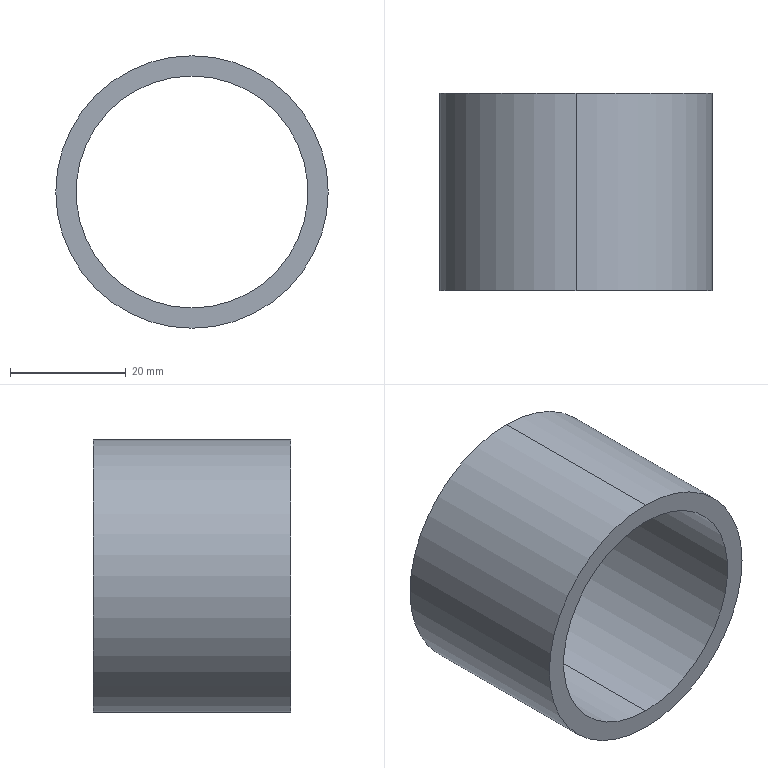Part | SolidWorks | features Extrusion 1 | 1 solid | 6 faces | box 47 x 34 x 47 mm | volume 16262 mm3 | cylinder 4 | plane 2 | commonest cylinder face diameters 40 x2 47 x2
STEP:
#1=CARTESIAN_POINT('',(0.,34.,-20.));
#2=VERTEX_POINT('',#1);
#3=CARTESIAN_POINT('',(0.,34.,20.));
#4=VERTEX_POINT('',#3);
#5=CARTESIAN_POINT('',(0.,34.,0.));
#6=DIRECTION('',(0.,1.,0.));
#7=DIRECTION('',(0.,0.,1.));
#8=AXIS2_PLACEMENT_3D('',#5,#6,#7);
#9=CIRCLE('',#8,20.);
#10=EDGE_CURVE('',#2,#4,#9,.T.);
#11=ORIENTED_EDGE('',*,*,#10,.T.);
#12=CARTESIAN_POINT('',(0.,0.,20.));
#13=VERTEX_POINT('',#12);
#14=CARTESIAN_POINT('',(0.,34.,20.));
#15=DIRECTION('',(0.,-1.,0.));
#16=VECTOR('',#15,1000.);
#17=LINE('',#14,#16);
#18=EDGE_CURVE('',#4,#13,#17,.T.);
#19=ORIENTED_EDGE('',*,*,#18,.T.);
#20=CARTESIAN_POINT('',(0.,0.,-20.));
#21=VERTEX_POINT('',#20);
#22=CARTESIAN_POINT('',(0.,0.,0.));
#23=DIRECTION('',(0.,1.,0.));
#24=DIRECTION('',(0.,0.,1.));
#25=AXIS2_PLACEMENT_3D('',#22,#23,#24);
#26=CIRCLE('',#25,20.);
#27=EDGE_CURVE('',#21,#13,#26,.T.);
#28=ORIENTED_EDGE('',*,*,#27,.F.);
#29=CARTESIAN_POINT('',(0.,34.,-20.));
#30=DIRECTION('',(0.,-1.,0.));
#31=VECTOR('',#30,1000.);
#32=LINE('',#29,#31);
#33=EDGE_CURVE('',#2,#21,#32,.T.);
#34=ORIENTED_EDGE('',*,*,#33,.F.);
#35=EDGE_LOOP('',(#11,#19,#28,#34));
#36=FACE_OUTER_BOUND('',#35,.T.);
#37=CARTESIAN_POINT('',(0.,34.,0.));
#38=DIRECTION('',(0.,-1.,0.));
#39=DIRECTION('',(0.,0.,-1.));
#40=AXIS2_PLACEMENT_3D('',#37,#38,#39);
#41=CYLINDRICAL_SURFACE('',#40,20.);
#42=ADVANCED_FACE('',(#36),#41,.F.);
#43=CARTESIAN_POINT('',(0.,34.,23.5));
#44=VERTEX_POINT('',#43);
#45=CARTESIAN_POINT('',(0.,34.,-23.5));
#46=VERTEX_POINT('',#45);
#47=CARTESIAN_POINT('',(0.,34.,0.));
#48=DIRECTION('',(0.,1.,0.));
#49=DIRECTION('',(0.,0.,1.));
#50=AXIS2_PLACEMENT_3D('',#47,#48,#49);
#51=CIRCLE('',#50,23.5);
#52=EDGE_CURVE('',#44,#46,#51,.T.);
#53=ORIENTED_EDGE('',*,*,#52,.F.);
#54=CARTESIAN_POINT('',(0.,0.,23.5));
#55=VERTEX_POINT('',#54);
#56=CARTESIAN_POINT('',(0.,34.,23.5));
#57=DIRECTION('',(0.,-1.,0.));
#58=VECTOR('',#57,1000.);
#59=LINE('',#56,#58);
#60=EDGE_CURVE('',#44,#55,#59,.T.);
#61=ORIENTED_EDGE('',*,*,#60,.T.);
#62=CARTESIAN_POINT('',(0.,0.,-23.5));
#63=VERTEX_POINT('',#62);
#64=CARTESIAN_POINT('',(0.,0.,0.));
#65=DIRECTION('',(0.,1.,0.));
#66=DIRECTION('',(0.,0.,1.));
#67=AXIS2_PLACEMENT_3D('',#64,#65,#66);
#68=CIRCLE('',#67,23.5);
#69=EDGE_CURVE('',#55,#63,#68,.T.);
#70=ORIENTED_EDGE('',*,*,#69,.T.);
#71=CARTESIAN_POINT('',(0.,34.,-23.5));
#72=DIRECTION('',(0.,-1.,0.));
#73=VECTOR('',#72,1000.);
#74=LINE('',#71,#73);
#75=EDGE_CURVE('',#46,#63,#74,.T.);
#76=ORIENTED_EDGE('',*,*,#75,.F.);
#77=EDGE_LOOP('',(#53,#61,#70,#76));
#78=FACE_OUTER_BOUND('',#77,.T.);
#79=CARTESIAN_POINT('',(0.,34.,0.));
#80=DIRECTION('',(0.,-1.,0.));
#81=DIRECTION('',(0.,0.,-1.));
#82=AXIS2_PLACEMENT_3D('',#79,#80,#81);
#83=CYLINDRICAL_SURFACE('',#82,23.5);
#84=ADVANCED_FACE('',(#78),#83,.T.);
#85=CARTESIAN_POINT('',(0.,34.,0.));
#86=DIRECTION('',(0.,1.,0.));
#87=DIRECTION('',(0.,0.,1.));
#88=AXIS2_PLACEMENT_3D('',#85,#86,#87);
#89=CIRCLE('',#88,23.5);
#90=EDGE_CURVE('',#46,#44,#89,.T.);
#91=ORIENTED_EDGE('',*,*,#90,.T.);
#92=ORIENTED_EDGE('',*,*,#52,.T.);
#93=EDGE_LOOP('',(#91,#92));
#94=FACE_OUTER_BOUND('',#93,.T.);
#95=ORIENTED_EDGE('',*,*,#10,.F.);
#96=CARTESIAN_POINT('',(0.,34.,0.));
#97=DIRECTION('',(0.,1.,0.));
#98=DIRECTION('',(0.,0.,1.));
#99=AXIS2_PLACEMENT_3D('',#96,#97,#98);
#100=CIRCLE('',#99,20.);
#101=EDGE_CURVE('',#4,#2,#100,.T.);
#102=ORIENTED_EDGE('',*,*,#101,.F.);
#103=EDGE_LOOP('',(#95,#102));
#104=FACE_BOUND('',#103,.T.);
#105=CARTESIAN_POINT('',(0.,34.,0.));
#106=DIRECTION('',(0.,1.,0.));
#107=DIRECTION('',(0.,0.,1.));
#108=AXIS2_PLACEMENT_3D('',#105,#106,#107);
#109=PLANE('',#108);
#110=ADVANCED_FACE('',(#94,#104),#109,.T.);
#111=CARTESIAN_POINT('',(0.,0.,0.));
#112=DIRECTION('',(0.,1.,0.));
#113=DIRECTION('',(0.,0.,1.));
#114=AXIS2_PLACEMENT_3D('',#111,#112,#113);
#115=CIRCLE('',#114,23.5);
#116=EDGE_CURVE('',#63,#55,#115,.T.);
#117=ORIENTED_EDGE('',*,*,#116,.F.);
#118=ORIENTED_EDGE('',*,*,#69,.F.);
#119=EDGE_LOOP('',(#117,#118));
#120=FACE_OUTER_BOUND('',#119,.T.);
#121=ORIENTED_EDGE('',*,*,#27,.T.);
#122=CARTESIAN_POINT('',(0.,0.,0.));
#123=DIRECTION('',(0.,1.,0.));
#124=DIRECTION('',(0.,0.,1.));
#125=AXIS2_PLACEMENT_3D('',#122,#123,#124);
#126=CIRCLE('',#125,20.);
#127=EDGE_CURVE('',#13,#21,#126,.T.);
#128=ORIENTED_EDGE('',*,*,#127,.T.);
#129=EDGE_LOOP('',(#121,#128));
#130=FACE_BOUND('',#129,.T.);
#131=CARTESIAN_POINT('',(0.,0.,0.));
#132=DIRECTION('',(0.,1.,0.));
#133=DIRECTION('',(0.,0.,1.));
#134=AXIS2_PLACEMENT_3D('',#131,#132,#133);
#135=PLANE('',#134);
#136=ADVANCED_FACE('',(#120,#130),#135,.F.);
#137=ORIENTED_EDGE('',*,*,#60,.F.);
#138=ORIENTED_EDGE('',*,*,#90,.F.);
#139=ORIENTED_EDGE('',*,*,#75,.T.);
#140=ORIENTED_EDGE('',*,*,#116,.T.);
#141=EDGE_LOOP('',(#137,#138,#139,#140));
#142=FACE_OUTER_BOUND('',#141,.T.);
#143=CARTESIAN_POINT('',(0.,34.,0.));
#144=DIRECTION('',(0.,-1.,0.));
#145=DIRECTION('',(0.,0.,-1.));
#146=AXIS2_PLACEMENT_3D('',#143,#144,#145);
#147=CYLINDRICAL_SURFACE('',#146,23.5);
#148=ADVANCED_FACE('',(#142),#147,.T.);
#149=ORIENTED_EDGE('',*,*,#18,.F.);
#150=ORIENTED_EDGE('',*,*,#101,.T.);
#151=ORIENTED_EDGE('',*,*,#33,.T.);
#152=ORIENTED_EDGE('',*,*,#127,.F.);
#153=EDGE_LOOP('',(#149,#150,#151,#152));
#154=FACE_OUTER_BOUND('',#153,.T.);
#155=CARTESIAN_POINT('',(0.,34.,0.));
#156=DIRECTION('',(0.,-1.,0.));
#157=DIRECTION('',(0.,0.,-1.));
#158=AXIS2_PLACEMENT_3D('',#155,#156,#157);
#159=CYLINDRICAL_SURFACE('',#158,20.);
#160=ADVANCED_FACE('',(#154),#159,.F.);
#161=CLOSED_SHELL('',(#42,#84,#110,#136,#148,#160));
#162=MANIFOLD_SOLID_BREP('',#161);
#163=CARTESIAN_POINT('',(0.,0.,0.));
#164=DIRECTION('',(0.,0.,1.));
#165=DIRECTION('',(1.,0.,0.));
#166=AXIS2_PLACEMENT_3D('',#163,#164,#165);
#167=(LENGTH_UNIT()NAMED_UNIT(*)SI_UNIT(.MILLI.,.METRE.));
#168=UNCERTAINTY_MEASURE_WITH_UNIT(LENGTH_MEASURE(0.00001),#167,'','');
#169=(NAMED_UNIT(*)PLANE_ANGLE_UNIT()SI_UNIT($,.RADIAN.));
#170=(NAMED_UNIT(*)SI_UNIT($,.STERADIAN.)SOLID_ANGLE_UNIT());
#171=(GEOMETRIC_REPRESENTATION_CONTEXT(3)GLOBAL_UNCERTAINTY_ASSIGNED_CONTEXT((#168))GLOBAL_UNIT_ASSIGNED_CONTEXT((#167,#169,#170))REPRESENTATION_CONTEXT('',''));
#172=ADVANCED_BREP_SHAPE_REPRESENTATION('',(#162,#166),#171);